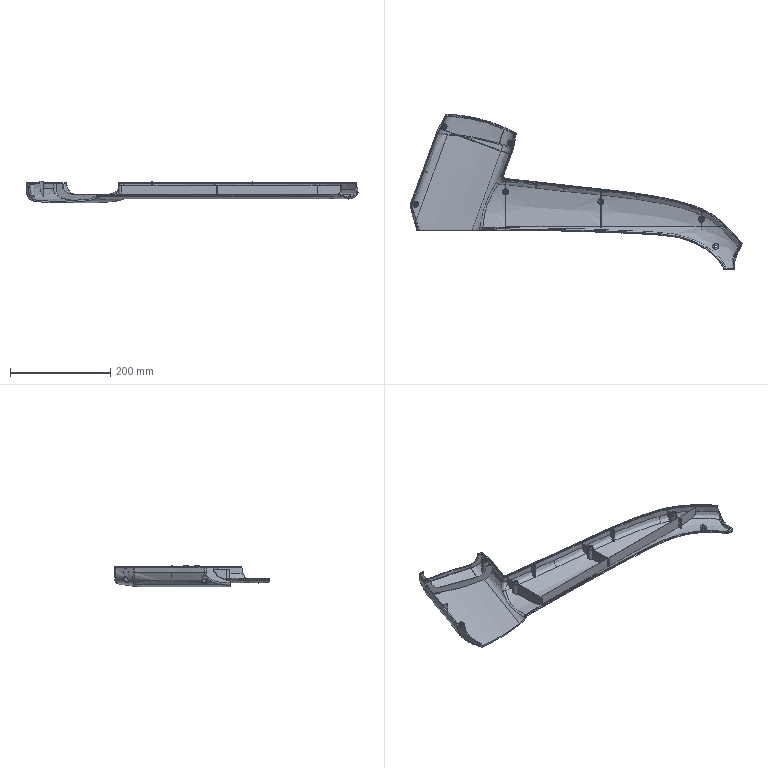Part | STEP file | PR12S0312~665.310.45LR | 1 solid | 275 faces | box 660.94 x 308.881 x 43 mm | volume 303745 mm3 | spline 112 | plane 95 | cylinder 65 | torus 3 | commonest cylinder face diameters 12 x12 8 x9 3.2 x6 8.5 x4 2 x3 5 x3